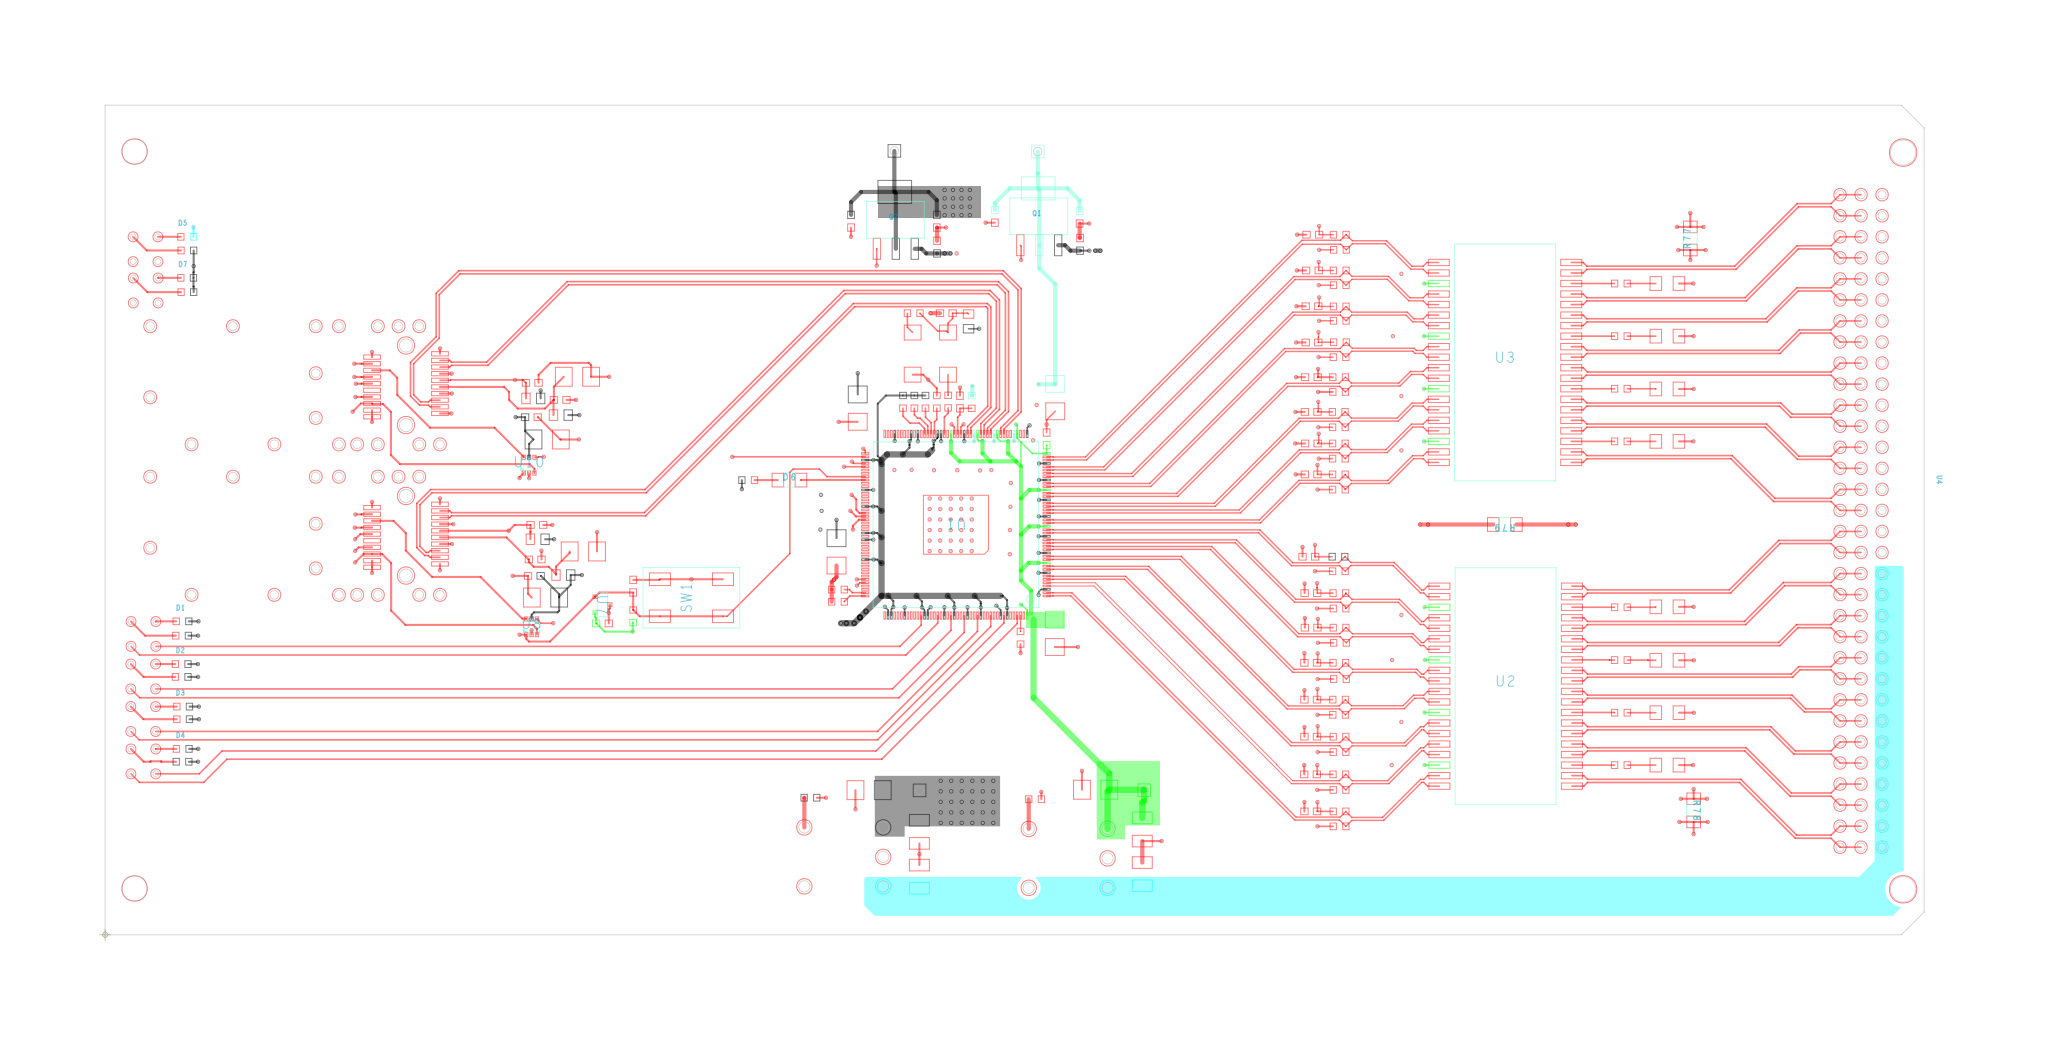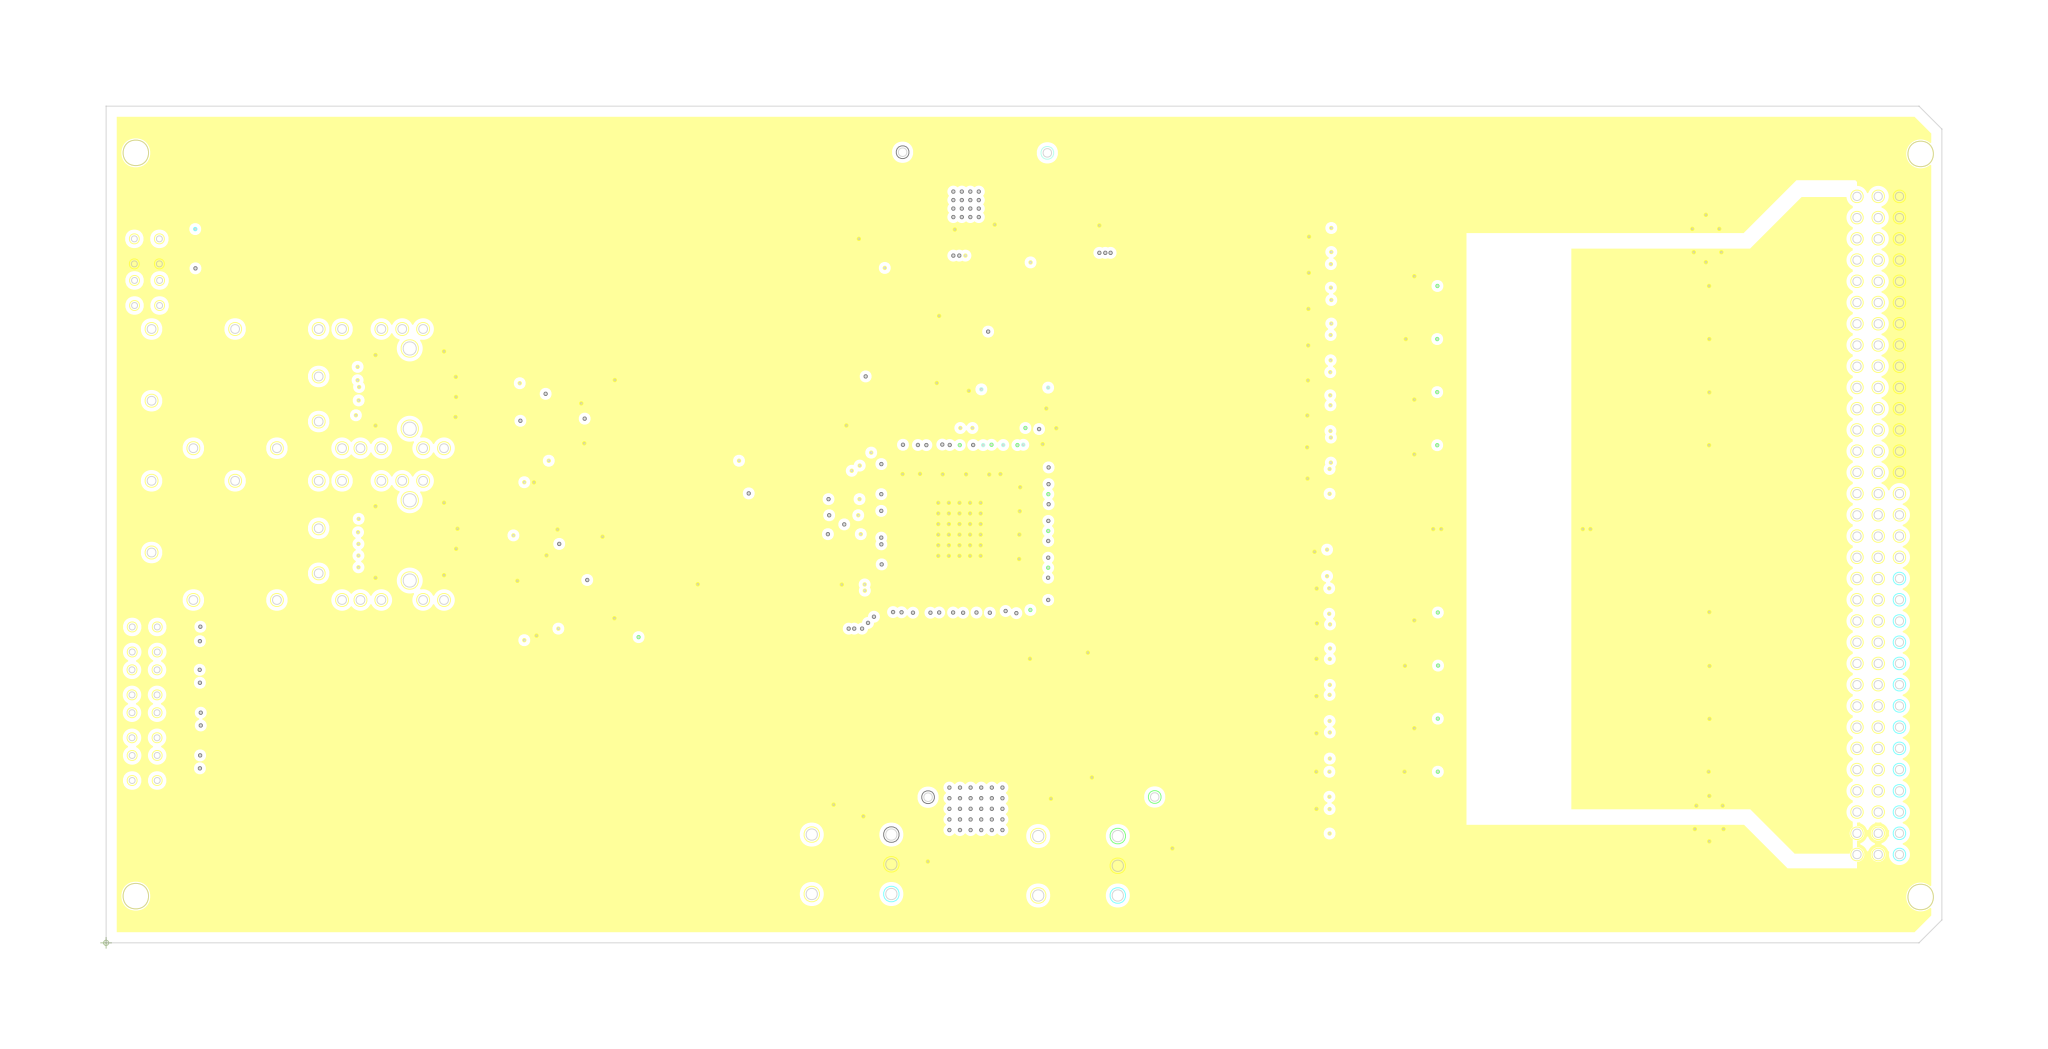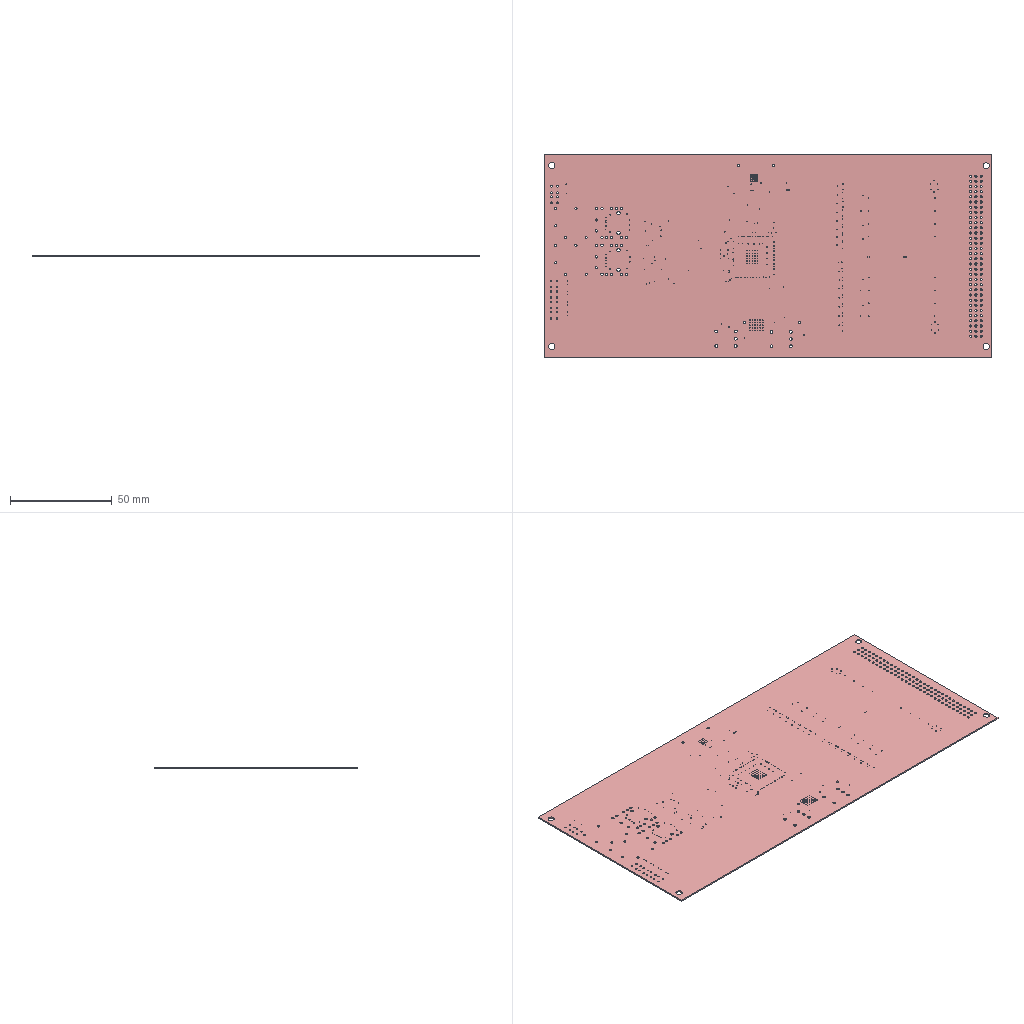Circuit board layout | Cadence Allegro | box 219.7 x 100.1 x 0.7 mm
Layer stack:
# Cadence Allegro layer stack of  (unit mm; from the constraint file cross-section; dielectric type: 0 not recorded (Allegro does not mark core vs prepreg), 3 surface material)
index,name,kind,layer,copper_thickness_mm,dielectric_type,dielectric_thickness_mm,dielectric_material,dielectric_constant
0,Top Surface,other,,,,,,
1,TOP,copper,TOP,0.0305,,,,
2,Dielectric1,dielectric,,,0,0.2032,FR-4,4.5
3,GND,copper,GND,0.0305,,,,
4,Dielectric2,dielectric,,,0,0.2032,FR-4,4.5
5,POWER,copper,POWER,0.0305,,,,
6,Dielectric3,dielectric,,,0,0.2032,FR-4,4.5
7,BOTTOM,copper,BOTTOM,0.0305,,,,
8,Bottom Surface,other,,,,,,
# drill layer pairs: low layer,high layer
drill_pair,TOP,BOTTOM
Part placement:
REFDES,COMP_VALUE,SYM_NAME,SYM_X,SYM_Y,SYM_ROTATE,SYM_MIRROR
+1.2V,T POINT R,TH,3753.00,3724.00,0.000,NO
+1.5V,T POINT R,TH,4435.00,3721.00,0.000,NO
+2.5V,T POINT R,TH,4941.00,687.00,0.000,NO
+3.3V,T POINT R,TH,3873.00,686.00,0.000,NO
C1,0.1uf,SC0603,5724.00,1796.00,0.000,NO
C2,0.1uf,SC0603,5734.00,1623.00,0.000,NO
C3,1NF-1000v,SC1206,7429.00,1558.00,180.000,NO
C4,0.1uf,SC0603,5735.00,1459.00,0.000,NO
C5,1NF-1000v,SC1206,7429.00,1304.00,180.000,NO
C6,0.1uf,SC0603,5733.00,1292.00,0.000,NO
C7,0.1uf,SC0603,5733.00,1117.00,0.000,NO
C8,1NF-1000v,SC1206,7429.00,1055.00,180.000,NO
C9,0.1uf,SC0603,5733.00,941.00,0.000,NO
C10,0.1uf,SC0603,5732.00,762.00,0.000,NO
C11,0.1uf,SC0603,5733.00,586.00,0.000,NO
C12,1NF-1000v,SC1206,7429.00,806.00,180.000,NO
C13,0.1uf,SC0603,6194.00,1556.00,0.000,YES
C14,0.1uf,SC0603,6194.00,1305.00,0.000,YES
C15,0.1uf,SC0603,6194.00,1056.00,0.000,YES
C16,0.1uf,SC0603,6194.00,806.00,0.000,YES
C17,0.1uf,SC0603,5743.00,3326.00,0.000,NO
C18,0.1uf,SC0603,5741.00,3156.00,0.000,NO
C19,1NF-1000v,SC1206,7429.00,3094.00,180.000,NO
C20,0.1uf,SC0603,5739.00,2986.00,0.000,NO
C21,1NF-1000v,SC1206,7429.00,2844.00,180.000,NO
C22,0.1uf,SC0603,5739.00,2814.00,0.000,NO
C23,0.1uf,SC0603,5736.00,2649.00,0.000,NO
C24,0.1uf,SC0603,5735.00,2484.00,0.000,NO
C25,1NF-1000v,SC1206,7429.00,2593.00,180.000,NO
C26,0.1uf,SC0603,5736.00,2334.00,0.000,NO
C27,1NF-1000v,SC1206,7429.00,2344.00,180.000,NO
C28,0.1uf,SC0603,5735.00,2187.00,0.000,NO
C29,0.1uf,SC0603,6194.00,3094.00,0.000,YES
C30,0.1uf,SC0603,6194.00,2844.00,0.000,YES
C31,0.1uf,SC0603,6194.00,2594.00,0.000,YES
C32,0.1uf,SC0603,6194.00,2345.00,0.000,YES
C33,0.1uf,SC0603,3690.00,2284.00,270.000,YES
C34,0.1uf,SC0603,3723.00,2032.00,180.000,YES
C35,0.1uf,SC0603,3725.00,1908.00,180.000,YES
C36,0.1uf,SC0603,3725.00,1777.00,180.000,YES
C37,0.1uf,SC0603,3882.00,1628.00,270.000,YES
C38,0.1uf,SC0603,4044.00,1628.00,270.000,YES
C39,0.1uf,SC0603,4160.00,1628.00,270.000,YES
C40,0.1uf,SC0603,4289.00,1628.00,270.000,YES
C41,0.1uf,SC0603,4379.00,2119.00,0.000,YES
C42,0.1uf,SC0603,4477.00,2356.00,90.000,NO
C43,0.1uf,SC0603,4186.00,2284.00,90.000,YES
C44,0.1uf,SC0603,4294.00,2284.00,90.000,YES
C45,10uF,STC3528,4516.00,1432.00,270.000,NO
C46,0.1uf,SC0603,3747.00,1628.00,270.000,YES
C47,0.1uf,SC0603,3806.00,2284.00,90.000,YES
C48,0.1uf,SC0603,3915.00,2284.00,90.000,YES
C49,10uF,STC3528,3478.00,1819.00,270.000,NO
C50,0.1uf,SC0603,4333.00,2487.00,270.000,YES
C51,0.1uf,SC0603,4377.00,1780.00,0.000,YES
C52,0.1uf,SC0603,4024.00,2284.00,90.000,YES
C53,0.1uf,SC0603,4377.00,1951.00,0.000,YES
C54,0.1uf,SC0603,4350.00,1628.00,270.000,YES
C55,0.1uf,SC0603,4133.00,2284.00,90.000,YES
C56,0.1uf,SC0603,4240.00,2284.00,90.000,YES
C57,0.1uf,SC0603,4383.00,2312.00,180.000,YES
C58,10uF,STC3528,4518.00,2552.00,270.000,NO
C59,0.1uf,SC0603,3753.00,2284.00,90.000,YES
C60,0.1uf,SC0603,3862.00,2284.00,90.000,YES
C61,0.1uf,SC0603,3970.00,2284.00,90.000,YES
C62,0.1uf,SC0603,4079.00,2284.00,90.000,YES
C63,0.1uf,SC0603,4388.00,2487.00,270.000,YES
C64,0.1uf,SC0603,4379.00,2240.00,0.000,YES
C65,0.1uf,SC0603,4379.00,2174.00,0.000,YES
C66,0.1uf,SC0603,4379.00,2063.00,0.000,YES
C67,0.1uf,SC0603,4378.00,2007.00,0.000,YES
C68,0.1uf,SC0603,4377.00,1895.00,0.000,YES
C69,0.1uf,SC0603,4377.00,1837.00,0.000,YES
C70,0.1uf,SC0603,4378.00,1721.00,0.000,YES
C71,0.1uf,SC0603,4409.00,1627.00,270.000,YES
C72,0.1uf,SC0603,4234.00,1628.00,270.000,YES
C73,0.1uf,SC0603,4098.00,1628.00,270.000,YES
C74,0.1uf,SC0603,3991.00,1628.00,270.000,YES
C75,0.1uf,SC0603,3936.00,1628.00,270.000,YES
C76,0.1uf,SC0603,3693.00,1628.00,270.000,YES
C77,0.1uf,SC0603,3803.00,1627.00,270.000,YES
C78,0.1uf,SC0603,3725.00,1853.00,180.000,YES
C79,0.1uf,SC0603,3724.00,2113.00,180.000,YES
C80,10uF,STC3528,3579.00,2502.00,270.000,NO
C81,0.1uf,SC0603,4065.00,2531.00,90.000,NO
C82,4.7U_10V_CER,SC0603,4636.00,3280.00,90.000,NO
C83,4.7U_10V_CER,SC0603,4634.00,3409.00,270.000,NO
C84,4.7U_10V_CER,SC0603,4231.00,3413.00,270.000,NO
C85,4.7U_10V_CER,SC0603,3956.00,3267.00,90.000,NO
C86,4.7U_10V_CER,SC0603,3955.00,3390.00,270.000,NO
C87,4.7U_10V_CER,SC0603,3547.00,3390.00,270.000,NO
C88,47uF,SC1210,3872.00,276.00,90.000,NO
C89,47uF,STC3528,3633.00,687.00,180.000,NO
C90,47uF,STC3528,4710.00,689.00,180.000,NO
C91,47uF,SC1210,3872.00,489.00,270.000,NO
C92,47uF,SC1210,4932.00,288.00,90.000,NO
C93,47uF,SC1210,4932.00,500.00,270.000,NO
C94,0.1uf,SC0603,2365.00,1479.00,0.000,NO
C95,470uF,SC0603,2511.00,1656.00,90.000,NO
C96,0.1uf,SC0603,4000.00,2953.00,0.000,NO
C97,0.1uf,SC0603,2027.00,2459.00,0.000,NO
C98,10uF,STC3528,2102.00,2353.00,0.000,NO
C99,0.1uf,SC0603,2031.00,2622.00,0.000,NO
C100,0.1uf,SC0603,2164.00,2541.00,0.000,NO
C101,10uF,STC3528,2246.00,2651.00,0.000,NO
C102,0.1uf,SC0603,2041.00,1705.00,180.000,NO
C103,10uF,STC3528,2094.00,1602.00,180.000,NO
C104,0.1uf,SC0603,2053.00,1947.00,0.000,NO
C105,0.1uf,SC0603,2045.00,1783.00,0.000,NO
C106,10uF,STC3528,2274.00,1821.00,0.000,NO
D1,LN02202_0,LED_2,123.00,1488.00,0.000,NO
D2,LN02202_0,LED_2,122.00,1286.00,0.000,NO
D3,LN02202_0,LED_2,122.00,1084.00,0.000,NO
D4,LN02202_0,LED_2,122.67,882.64,0.000,NO
D5,LN02202_0,LED_2,133.00,3316.00,0.000,NO
D6,LED,SD1206,3254.00,2160.00,0.000,NO
D7,LN02202_0,LED_2,134.00,3120.00,0.000,NO
L1,1200HM,SL0805,4106.00,2914.00,270.000,NO
L2,1200HM,SL0805,2036.00,2548.00,180.000,NO
L3,1200HM,SL0805,2057.00,1879.00,180.000,NO
L4,1200HM,SL0805,2167.00,2469.00,180.000,NO
L5,1200HM,SL0805,2179.00,1709.00,180.000,NO
Q1,BCP69T1,SOT223,4307.00,3381.00,90.000,NO
Q2,BCP69T1,SOT223,3625.00,3364.00,90.000,NO
R1,49.9,SR0603,5865.00,1796.00,0.000,NO
R2,49.9,SR0603,5867.00,1727.00,0.000,NO
R3,49.9,SR0603,5869.00,1623.00,0.000,NO
R4,75,SR0603,7208.00,1556.00,0.000,NO
R5,49.9,SR0603,5870.00,1550.00,0.000,NO
R6,49.9,SR0603,5870.00,1459.00,0.000,NO
R7,49.9,SR0603,5872.00,1387.00,0.000,NO
R8,49.9,SR0603,5869.00,1292.00,0.000,NO
R9,75,SR0603,7208.00,1305.00,0.000,NO
R10,49.9,SR0603,5872.00,1215.00,0.000,NO
R11,49.9,SR0603,5868.00,1117.00,0.000,NO
R12,49.9,SR0603,5868.00,1045.00,0.000,NO
R13,75,SR0603,7208.00,1055.00,0.000,NO
R14,49.9,SR0603,5870.00,941.00,0.000,NO
R15,49.9,SR0603,5870.00,868.00,0.000,NO
R16,49.9,SR0603,5869.00,762.00,0.000,NO
R17,49.9,SR0603,5870.00,688.00,0.000,NO
R18,49.9,SR0603,5870.00,586.00,0.000,NO
R19,75,SR0603,7208.00,806.00,0.000,NO
R20,49.9,SR0603,5870.00,515.00,0.000,NO
R21,49.9,SR0603,5871.00,3326.00,0.000,NO
R22,49.9,SR0603,5872.00,3254.00,0.000,NO
R23,75,SR0603,7208.00,3094.00,0.000,NO
R24,49.9,SR0603,5871.00,3156.00,0.000,NO
R25,49.9,SR0603,5871.00,3086.00,0.000,NO
R26,49.9,SR0603,5871.00,2985.00,0.000,NO
R27,49.9,SR0603,5871.00,2917.00,0.000,NO
R28,75,SR0603,7208.00,2844.00,0.000,NO
R29,49.9,SR0603,5872.00,2815.00,0.000,NO
R30,49.9,SR0603,5870.00,2744.00,0.000,NO
R31,49.9,SR0603,5868.00,2649.00,0.000,NO
R32,49.9,SR0603,5868.00,2579.00,0.000,NO
R33,49.9,SR0603,5866.00,2484.00,0.000,NO
R34,75,SR0603,7208.00,2594.00,0.000,NO
R35,49.9,SR0603,5867.00,2411.00,0.000,NO
R36,49.9,SR0603,5867.00,2334.00,0.000,NO
R37,49.9,SR0603,5867.00,2262.00,0.000,NO
R38,75,SR0603,7208.00,2344.00,0.000,NO
R39,49.9,SR0603,5867.00,2187.00,0.000,NO
R40,49.9,SR0603,5867.00,2115.00,0.000,NO
R41,0,SR0603,4121.00,2531.00,270.000,NO
R42,330ohm,SR0603,368.00,1489.00,0.000,NO
R43,330ohm,SR0603,366.00,1421.00,0.000,NO
R44,330ohm,SR0603,364.00,1286.00,0.000,NO
R45,330ohm,SR0603,364.00,1225.00,0.000,NO
R46,330ohm,SR0603,371.00,1084.00,0.000,NO
R47,330ohm,SR0603,371.00,1024.00,0.000,NO
R48,330ohm,SR0603,369.00,883.00,0.000,NO
R49,330ohm,SR0603,368.00,822.00,0.000,NO
R50,4.7K,SR0603,3794.00,2532.00,270.000,NO
R51,4.7K_NOB,SR0603,3848.00,2532.00,270.000,NO
R52,4.7K,SR0603,3901.00,2532.00,270.000,NO
R53,O_NOB,SR0603,3955.00,2532.00,90.000,NO
R54,475ohm-1%,SR0603,3354.00,651.00,0.000,NO
R55,2.32K-1%,SR0603,4422.00,644.00,0.000,NO
R56,330ohm,SR0603,390.00,3316.00,0.000,NO
R57,330ohm,SR0603,391.00,3251.00,0.000,NO
R58,150ohm,SR0603,3058.00,2160.00,0.000,NO
R59,1K,SR0603,2511.00,1513.00,90.000,NO
R60,0ohm_NOB,SR0603,3485.00,1640.00,0.000,NO
R61,0ohm,SR0603,3485.00,1582.00,0.000,NO
R62,2K_1%,SR0603,4353.00,1411.00,270.000,NO
R63,4.7K,SR0603,3845.00,2953.00,180.000,NO
R64,22ohm,SR0603,4009.00,2533.00,270.000,NO
R65,330ohm,SR0603,390.00,3121.00,0.000,NO
R66,330ohm,SR0603,391.00,3053.00,0.000,NO
R67,4.7K,SR0603,1114.00,2540.00,180.000,YES
R68,4.7K,SR0603,1114.00,2650.00,180.000,YES
R69,4.7K,SR0603,1114.00,2595.00,180.000,YES
R70,4.7K,SR0603,1115.00,2713.00,180.000,YES
R71,4.7K,SR0603,1114.00,2485.00,180.000,YES
R72,4.7K,SR0603,1123.00,1824.00,180.000,YES
R73,4.7K,SR0603,1123.00,1934.00,180.000,YES
R74,4.7K,SR0603,1123.00,1879.00,180.000,YES
R75,4.7K,SR0603,1123.00,1997.00,180.000,YES
R76,4.7K,SR0603,1123.00,1769.00,180.000,YES
R77,R,SD1206,7538.00,3308.00,90.000,NO
R78,R,SD1206,7554.00,591.00,270.000,NO
R79,R,SD1206,6656.00,1949.00,180.000,NO
R80,4.7K,SR0603,3479.00,1925.00,180.000,YES
R81,4.7K_NOB,SR0603,3479.00,2014.00,180.000,YES
R82,4.7K,SR0603,3479.00,2090.00,180.000,YES
SW1,SW_4,SW-4,2788.00,1601.00,90.000,NO
TP1,T POINT R,HOLE27-6AA,140.00,3721.00,0.000,NO
TP2,T POINT R,HOLE27-6AA,140.00,220.00,0.000,NO
U1,88E6095,88E6097,4046.00,1948.00,90.000,NO
U2,HX1234,SO-40,6660.00,1181.00,0.000,NO
U3,HX1234,SO-40,6657.00,2719.00,0.000,NO
U4,Jack_32*3,CON96,7983.00,123.00,270.000,NO
U5,PTH04070W,PTH04070W,3780.00,590.00,180.000,NO
U6,PTH04070W,PTH04070W,4847.00,583.00,180.000,NO
U7,MXD1818UR22-T,SOT23,2365.00,1569.00,0.000,NO
U8,NC7WZ14,NC7W14,2028.00,1463.00,0.000,NO
U9,SFP_HOST,SFPSHELL,1682.00,1533.00,90.000,NO
U10,NC7WZ14,NC7W14,2016.00,2231.00,0.000,NO
U11,SFP_HOST,SFPSHELL,1682.00,2248.00,90.000,NO
X1,25MHz,SX4-0805A,3909.00,2761.00,270.000,NO
Pad and via stacks:
# Allegro (Cadence) via spans and padstacks; design units: ("mils" 2 100)
# via spans: padstack,start_layer,end_layer,net_example,count
VIA_BGA,ETCH/TOP,ETCH/BOTTOM,+3.3V,325
# Allegro padstack definitions: name,start_layer,end_layer,drill,plating,holeType,type
SMD35_32,"ETCH/TOP","ETCH/TOP",0.0,"PLATED","none","smd"
SMD80_90,"ETCH/TOP","ETCH/TOP",0.0,"PLATED","none","smd"
SMD55_65,"ETCH/TOP","ETCH/TOP",0.0,"PLATED","none","smd"
SMD55_95,"ETCH/TOP","ETCH/TOP",0.0,"PLATED","none","smd"
SMD40_50,"ETCH/TOP","ETCH/TOP",0.0,"PLATED","none","smd"
SMD160_110,"ETCH/TOP","ETCH/TOP",0.0,"PLATED","none","smd"
SMD100REC35,"ETCH/TOP","ETCH/TOP",0.0,"PLATED","none","smd"
SMD30_32,"ETCH/TOP","ETCH/TOP",0.0,"PLATED","none","smd"
R787_711C50,"ETCH/TOP","ETCH/TOP",0.0,"PLATED","none","smd"
R87_20,"ETCH/TOP","ETCH/TOP",0.0,"PLATED","none","smd"
R50_40,"ETCH/TOP","ETCH/TOP",0.0,"PLATED","none","smd"
SMD100_30,"ETCH/TOP","ETCH/TOP",0.0,"PLATED","none","smd"
SMD20_17,"ETCH/TOP","ETCH/TOP",0.0,"PLATED","none","smd"
SFP2,"ETCH/TOP","ETCH/TOP",0.0,"PLATED","none","smd"
SMD71_80,"ETCH/TOP","ETCH/TOP",0.0,"PLATED","none","smd"
HOLE28,"ETCH/TOP","ETCH/BOTTOM",28.0,"PLATED","circle_drill","through"
PAD80CIR65D,"ETCH/TOP","ETCH/BOTTOM",66.0,"PLATED","circle_drill","through"
PAD55CIR40D,"ETCH/TOP","ETCH/BOTTOM",40.0,"PLATED","circle_drill","through"
PAD55SQ40,"ETCH/TOP","ETCH/BOTTOM",40.0,"PLATED","circle_drill","through"
HOLE120_DIP,"ETCH/TOP","ETCH/BOTTOM",120.0,"PLATED","circle_drill","through"
HOLE120,"ETCH/TOP","ETCH/BOTTOM",120.0,"PLATED","circle_drill","through"
HOLE40,"ETCH/TOP","ETCH/BOTTOM",39.0,"PLATED","circle_drill","through"
HOLE54,"ETCH/TOP","ETCH/BOTTOM",53.0,"PLATED","circle_drill","through"
SFPVIA2,"ETCH/TOP","ETCH/BOTTOM",62.0,"PLATED","circle_drill","through"
VIA61_3D41_3,"ETCH/TOP","ETCH/BOTTOM",41.3,"PLATED","circle_drill","through"
VIA_BGA,"ETCH/TOP","ETCH/BOTTOM",8.0,"PLATED","circle_drill","through"
SMD60_100,"ETCH/TOP","ETCH/TOP",0.0,"PLATED","none","smd"
Design rules, without the lines most boards share, first 11 of 60 lines:
# Cadence Allegro design rules of  (from the Constraint Manager export constraints.dcfx, design unit mil; typed fields in mm)
# columns: name | kind | enabled | priority | scope1 | scope2 | descriptor | typed fields (field=value)
# Allegro precedence (priority 1 wins): 1 Region class-to-class, 2 Region class, 3 Region, 4 class-to-class, 5 DiffPair/Bus/NetGroup override, 6 NetClass, 7 constraint set (CSet) default
# per-layer values are written LAYER=value in the descriptor and LAYER:mm in the typed field; a maximum of 0 means no limit set
# --- net classes (and buses / net groups) ---
DIFF | NetClass | enabled | 6 | RD0, RD1, RD2, RD3, RD4, RD5, RD6, RD7, RD9, TD0, TD1, TD2, TD3, TD4, TD5, TD6, TD7, TD9 | All | Net Class (ElectricalCSet=DIFF) (members: 18 DiffPair) overrides: (DIFFP_MIN_SPACE=4mil) | electricalcset=DIFF diffp_min_space=0.1016
# --- track widths, neck and differential-pair gap (physical constraint sets) ---
DEFAULT | PhysicalCSet | enabled | 7 | Design default | All | Physical Constraint (Min Line Width=5mil) (Max Line Width=30mil) (Min Neck Width=5mil) (Max Neck Length=0mil) (DiffPair Primary Gap=0mil) (DiffPair Neck Gap=0mil) (DiffPair Min Space=0mil) (DiffPair Coupled +Tol=0mil) (DiffPair Coupled -Tol=0mil) (Min BB Via Stagger=5mil) (Max BB Via Stagger=0mil) (T-junctions=ANYWHERE) (Pad-pad direct connect=ALL_ALLOWED) (Allowed vias=VIA_BGA) | min_line_width=0.127 min_neck_width=0.127 min_bvia_stagger=0.127 max_bvia_stagger=0 ts_allowed=ANYWHERE diffp_primary_gap=0 diffp_neck_gap=0 max_line_width=0.762 maximum_neck_length=0 pad_pad_direct_connect=ALL_ALLOWED allow_on_etch_subclass=TRUE diffp_coupled_plus=0 diffp_coupled_minus=0 diffp_min_space=0 vias=VIA_BGA
# --- clearances: line / pad / via / shape / hole (spacing constraint sets) ---
DEFAULT | SpacingCSet | enabled | 7 | Design default | All | Clearance Constraint (Line-Line=5mil) (Line-SMD Pad=5mil) (Line-Thru Pin=5mil) (Line-Via=5mil) (Line-Shape=20mil) (SMD Pad-SMD Pad=5mil) (Thru Pin-Thru Pin=5mil) (Thru Pin-SMD Pad=5mil) (SMD Pad-Via=5mil) (Thru Pin-Via=5mil) (Via-Via=5mil) (Shape-SMD Pad=7mil) (Shape-Thru Pin=20mil) (Shape-Via=20mil) (Shape-Shape=20mil) (Hole-Hole=8mil) (Hole-Line=8mil) (Hole-Shape=8mil) (BB Via-BB Via=5mil) (uVia-uVia=5mil) | thrupin_to_thrupin_spacing=0.127 thrupin_to_smdpin_spacing=0.127 thrupin_to_thruvia_spacing=0.127 line_to_thrupin_spacing=0.127 thrupin_to_shape_spacing=0.508 smdpin_to_smdpin_spacing=0.127 smdpin_to_thruvia_spacing=0.127 line_to_smdpin_spacing=0.127 shape_to_smdpin_spacing=0.1778 thruvia_to_thruvia_spacing=0.127 line_to_thruvia_spacing=0.127 shape_to_thruvia_spacing=0.508 line_to_line_spacing=0.127 line_to_shape_spacing=0.508 shape_to_shape_spacing=0.508 bbv_to_bbv_spacing=0.127 bbv_to_thrupin_spacing=0.127 bbv_to_smdpin_spacing=0.127 bbv_to_thruvia_spacing=0.127 bbv_to_line_spacing=0.127 bbv_to_shape_spacing=0.508 bbv_to_testpin_spacing=0.127 bbv_to_testvia_spacing=0.127 testpin_to_testpin_spacing=0.127 testpin_to_thrupin_spacing=0.127 smdpin_to_testpin_spacing=0.127 testpin_to_thruvia_spacing=0.127 testpin_to_testvia_spacing=0.127 line_to_testpin_spacing=0.127 shape_to_testpin_spacing=0.508 testvia_to_testvia_spacing=0.127 testvia_to_thrupin_spacing=0.127 smdpin_to_testvia_spacing=0.127 testvia_to_thruvia_spacing=0.127 line_to_testvia_spacing=0.127 shape_to_testvia_spacing=0.508 bondpad_to_bondpad_spacing=0.127 thrupin_to_bondpad_spacing=0.127 smdpin_to_bondpad_spacing=0.127 bondpad_to_thruvia_spacing=0.127 bondpad_to_line_spacing=0.127 bondpad_to_shape_spacing=0.508 bondpad_to_bbv_spacing=0.127 bondpad_to_testpin_spacing=0.127 bondpad_to_testvia_spacing=0.127 hole_to_pin_spacing=0.2032 hole_to_via_spacing=0.2032 hole_to_line_spacing=0.2032 hole_to_shape_spacing=0.2032 hole_to_hole_spacing=0.2032 mvia_to_mvia_spacing=0.127 mvia_to_thrupin_spacing=0.127 mvia_to_smdpin_spacing=0.127 mvia_to_thruvia_spacing=0.127 mvia_to_bbv_spacing=0.127 mvia_to_line_spacing=0.127 mvia_to_shape_spacing=0.127 mvia_to_testpin_spacing=0.127 mvia_to_testvia_spacing=0.127 bondpad_to_mvia_spacing=0.127 bondpad_to_bondpad_diffp_spc=0.127 min_bvia_gap=0.127
DIFFS | SpacingCSet | enabled | 7 | DiffPair(21): RD0, RD1, RD2, RD3, RD4, RD5, RD6, RD7, RD9, TD0, TD1, TD2, ... | All | Clearance Constraint (Line-Line=7mil) (Line-SMD Pad=7mil) (Line-Thru Pin=7mil) (Line-Via=7mil) (Line-Shape=7mil) (SMD Pad-SMD Pad=5mil) (Thru Pin-Thru Pin=5mil) (Thru Pin-SMD Pad=5mil) (SMD Pad-Via=5mil) (Thru Pin-Via=5mil) (Via-Via=5mil) (Shape-SMD Pad=5mil) (Shape-Thru Pin=5mil) (Shape-Via=5mil) (Shape-Shape=5mil) (Hole-Hole=8mil) (Hole-Line=7mil) (Hole-Shape=8mil) (BB Via-BB Via=5mil) (uVia-uVia=5mil) | bondpad_to_bondpad_diffp_spc=0.127 thrupin_to_thrupin_spacing=0.127 thrupin_to_smdpin_spacing=0.127 thrupin_to_thruvia_spacing=0.127 line_to_thrupin_spacing=0.1778 thrupin_to_shape_spacing=0.127 smdpin_to_smdpin_spacing=0.127 smdpin_to_thruvia_spacing=0.127 line_to_smdpin_spacing=0.1778 shape_to_smdpin_spacing=0.127 thruvia_to_thruvia_spacing=0.127 line_to_thruvia_spacing=0.1778 shape_to_thruvia_spacing=0.127 line_to_line_spacing=0.1778 line_to_shape_spacing=0.1778 shape_to_shape_spacing=0.127 bbv_to_bbv_spacing=0.127 bbv_to_thrupin_spacing=0.127 bbv_to_smdpin_spacing=0.127 bbv_to_thruvia_spacing=0.127 bbv_to_line_spacing=0.1778 bbv_to_shape_spacing=0.127 bbv_to_testpin_spacing=0.127 bbv_to_testvia_spacing=0.127 testpin_to_testpin_spacing=0.127 testpin_to_thrupin_spacing=0.127 smdpin_to_testpin_spacing=0.127 testpin_to_thruvia_spacing=0.127 testpin_to_testvia_spacing=0.127 line_to_testpin_spacing=0.1778 shape_to_testpin_spacing=0.127 testvia_to_testvia_spacing=0.127 testvia_to_thrupin_spacing=0.127 smdpin_to_testvia_spacing=0.127 testvia_to_thruvia_spacing=0.127 line_to_testvia_spacing=0.1778 shape_to_testvia_spacing=0.127 bondpad_to_bondpad_spacing=0.127 thrupin_to_bondpad_spacing=0.127 smdpin_to_bondpad_spacing=0.127 bondpad_to_thruvia_spacing=0.127 bondpad_to_line_spacing=0.1778 bondpad_to_shape_spacing=0.127 bondpad_to_bbv_spacing=0.127 bondpad_to_testpin_spacing=0.127 bondpad_to_testvia_spacing=0.127 hole_to_pin_spacing=0.2032 hole_to_via_spacing=0.2032 hole_to_line_spacing=0.1778 hole_to_shape_spacing=0.2032 hole_to_hole_spacing=0.2032 mvia_to_mvia_spacing=0.127 mvia_to_thrupin_spacing=0.127 mvia_to_smdpin_spacing=0.127 mvia_to_thruvia_spacing=0.127 mvia_to_bbv_spacing=0.127 mvia_to_line_spacing=0.127 mvia_to_shape_spacing=0.127 mvia_to_testpin_spacing=0.127 mvia_to_testvia_spacing=0.127 bondpad_to_mvia_spacing=0.127 min_bvia_gap=0.127